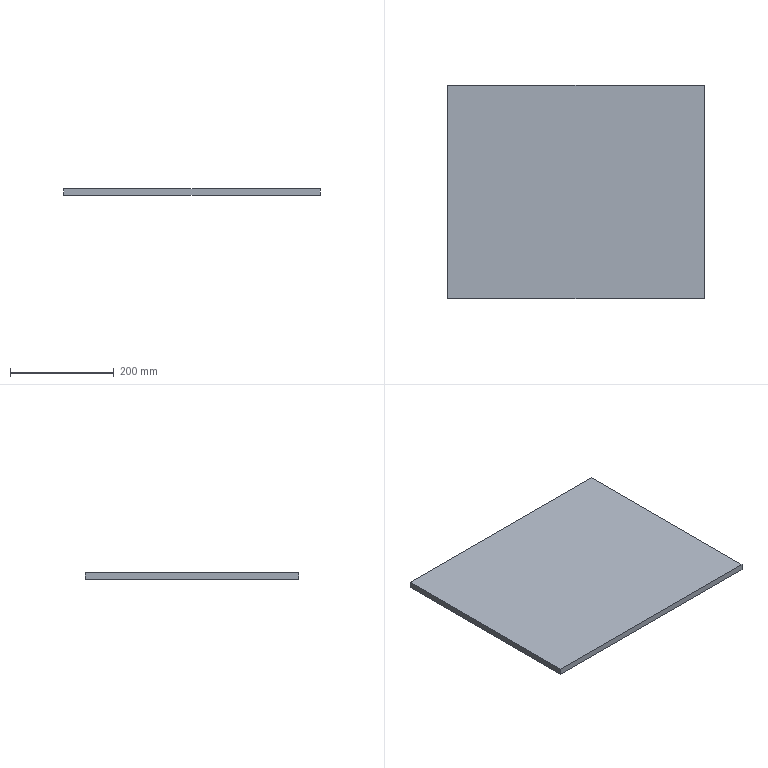Part | STEP file | Guide rail mounting plate | 1 solid | 6 faces | box 493 x 410 x 12 mm | volume 2425560 mm3 | plane 6
STEP:
#1=CARTESIAN_POINT('',(246.5,-205.,0.));
#2=VERTEX_POINT('',#1);
#3=CARTESIAN_POINT('',(246.5,205.,0.));
#4=VERTEX_POINT('',#3);
#5=CARTESIAN_POINT('',(246.5,-205.,0.));
#6=DIRECTION('',(0.,1.,0.));
#7=VECTOR('',#6,1000.);
#8=LINE('',#5,#7);
#9=EDGE_CURVE('',#2,#4,#8,.T.);
#10=ORIENTED_EDGE('',*,*,#9,.T.);
#11=CARTESIAN_POINT('',(246.5,205.,12.));
#12=VERTEX_POINT('',#11);
#13=CARTESIAN_POINT('',(246.5,205.,12.));
#14=DIRECTION('',(0.,0.,-1.));
#15=VECTOR('',#14,1000.);
#16=LINE('',#13,#15);
#17=EDGE_CURVE('',#12,#4,#16,.T.);
#18=ORIENTED_EDGE('',*,*,#17,.F.);
#19=CARTESIAN_POINT('',(246.5,-205.,12.));
#20=VERTEX_POINT('',#19);
#21=CARTESIAN_POINT('',(246.5,-205.,12.));
#22=DIRECTION('',(0.,1.,0.));
#23=VECTOR('',#22,1000.);
#24=LINE('',#21,#23);
#25=EDGE_CURVE('',#20,#12,#24,.T.);
#26=ORIENTED_EDGE('',*,*,#25,.F.);
#27=CARTESIAN_POINT('',(246.5,-205.,12.));
#28=DIRECTION('',(0.,0.,-1.));
#29=VECTOR('',#28,1000.);
#30=LINE('',#27,#29);
#31=EDGE_CURVE('',#20,#2,#30,.T.);
#32=ORIENTED_EDGE('',*,*,#31,.T.);
#33=EDGE_LOOP('',(#10,#18,#26,#32));
#34=FACE_OUTER_BOUND('',#33,.T.);
#35=CARTESIAN_POINT('',(246.5,-205.,12.));
#36=DIRECTION('',(-1.,0.,0.));
#37=DIRECTION('',(0.,0.,1.));
#38=AXIS2_PLACEMENT_3D('',#35,#36,#37);
#39=PLANE('',#38);
#40=ADVANCED_FACE('',(#34),#39,.F.);
#41=CARTESIAN_POINT('',(-246.5,205.,0.));
#42=VERTEX_POINT('',#41);
#43=CARTESIAN_POINT('',(-246.5,205.,0.));
#44=DIRECTION('',(-1.,0.,0.));
#45=VECTOR('',#44,1000.);
#46=LINE('',#43,#45);
#47=EDGE_CURVE('',#4,#42,#46,.T.);
#48=ORIENTED_EDGE('',*,*,#47,.T.);
#49=CARTESIAN_POINT('',(-246.5,205.,12.));
#50=VERTEX_POINT('',#49);
#51=CARTESIAN_POINT('',(-246.5,205.,12.));
#52=DIRECTION('',(0.,0.,-1.));
#53=VECTOR('',#52,1000.);
#54=LINE('',#51,#53);
#55=EDGE_CURVE('',#50,#42,#54,.T.);
#56=ORIENTED_EDGE('',*,*,#55,.F.);
#57=CARTESIAN_POINT('',(-246.5,205.,12.));
#58=DIRECTION('',(-1.,0.,0.));
#59=VECTOR('',#58,1000.);
#60=LINE('',#57,#59);
#61=EDGE_CURVE('',#12,#50,#60,.T.);
#62=ORIENTED_EDGE('',*,*,#61,.F.);
#63=ORIENTED_EDGE('',*,*,#17,.T.);
#64=EDGE_LOOP('',(#48,#56,#62,#63));
#65=FACE_OUTER_BOUND('',#64,.T.);
#66=CARTESIAN_POINT('',(-246.5,205.,12.));
#67=DIRECTION('',(0.,-1.,0.));
#68=DIRECTION('',(0.,0.,-1.));
#69=AXIS2_PLACEMENT_3D('',#66,#67,#68);
#70=PLANE('',#69);
#71=ADVANCED_FACE('',(#65),#70,.F.);
#72=CARTESIAN_POINT('',(-246.5,-205.,0.));
#73=VERTEX_POINT('',#72);
#74=CARTESIAN_POINT('',(-246.5,-205.,0.));
#75=DIRECTION('',(0.,-1.,0.));
#76=VECTOR('',#75,1000.);
#77=LINE('',#74,#76);
#78=EDGE_CURVE('',#42,#73,#77,.T.);
#79=ORIENTED_EDGE('',*,*,#78,.T.);
#80=CARTESIAN_POINT('',(-246.5,-205.,12.));
#81=VERTEX_POINT('',#80);
#82=CARTESIAN_POINT('',(-246.5,-205.,12.));
#83=DIRECTION('',(0.,0.,-1.));
#84=VECTOR('',#83,1000.);
#85=LINE('',#82,#84);
#86=EDGE_CURVE('',#81,#73,#85,.T.);
#87=ORIENTED_EDGE('',*,*,#86,.F.);
#88=CARTESIAN_POINT('',(-246.5,-205.,12.));
#89=DIRECTION('',(0.,-1.,0.));
#90=VECTOR('',#89,1000.);
#91=LINE('',#88,#90);
#92=EDGE_CURVE('',#50,#81,#91,.T.);
#93=ORIENTED_EDGE('',*,*,#92,.F.);
#94=ORIENTED_EDGE('',*,*,#55,.T.);
#95=EDGE_LOOP('',(#79,#87,#93,#94));
#96=FACE_OUTER_BOUND('',#95,.T.);
#97=CARTESIAN_POINT('',(-246.5,-205.,12.));
#98=DIRECTION('',(1.,0.,0.));
#99=DIRECTION('',(0.,0.,-1.));
#100=AXIS2_PLACEMENT_3D('',#97,#98,#99);
#101=PLANE('',#100);
#102=ADVANCED_FACE('',(#96),#101,.F.);
#103=CARTESIAN_POINT('',(-246.5,-205.,0.));
#104=DIRECTION('',(1.,0.,0.));
#105=VECTOR('',#104,1000.);
#106=LINE('',#103,#105);
#107=EDGE_CURVE('',#73,#2,#106,.T.);
#108=ORIENTED_EDGE('',*,*,#107,.T.);
#109=ORIENTED_EDGE('',*,*,#31,.F.);
#110=CARTESIAN_POINT('',(-246.5,-205.,12.));
#111=DIRECTION('',(1.,0.,0.));
#112=VECTOR('',#111,1000.);
#113=LINE('',#110,#112);
#114=EDGE_CURVE('',#81,#20,#113,.T.);
#115=ORIENTED_EDGE('',*,*,#114,.F.);
#116=ORIENTED_EDGE('',*,*,#86,.T.);
#117=EDGE_LOOP('',(#108,#109,#115,#116));
#118=FACE_OUTER_BOUND('',#117,.T.);
#119=CARTESIAN_POINT('',(-246.5,-205.,12.));
#120=DIRECTION('',(0.,1.,0.));
#121=DIRECTION('',(0.,0.,1.));
#122=AXIS2_PLACEMENT_3D('',#119,#120,#121);
#123=PLANE('',#122);
#124=ADVANCED_FACE('',(#118),#123,.F.);
#125=ORIENTED_EDGE('',*,*,#25,.T.);
#126=ORIENTED_EDGE('',*,*,#61,.T.);
#127=ORIENTED_EDGE('',*,*,#92,.T.);
#128=ORIENTED_EDGE('',*,*,#114,.T.);
#129=EDGE_LOOP('',(#125,#126,#127,#128));
#130=FACE_OUTER_BOUND('',#129,.T.);
#131=CARTESIAN_POINT('',(0.,0.,12.));
#132=DIRECTION('',(0.,0.,-1.));
#133=DIRECTION('',(-1.,0.,0.));
#134=AXIS2_PLACEMENT_3D('',#131,#132,#133);
#135=PLANE('',#134);
#136=ADVANCED_FACE('',(#130),#135,.F.);
#137=ORIENTED_EDGE('',*,*,#9,.F.);
#138=ORIENTED_EDGE('',*,*,#107,.F.);
#139=ORIENTED_EDGE('',*,*,#78,.F.);
#140=ORIENTED_EDGE('',*,*,#47,.F.);
#141=EDGE_LOOP('',(#137,#138,#139,#140));
#142=FACE_OUTER_BOUND('',#141,.T.);
#143=CARTESIAN_POINT('',(0.,0.,0.));
#144=DIRECTION('',(0.,0.,-1.));
#145=DIRECTION('',(-1.,0.,0.));
#146=AXIS2_PLACEMENT_3D('',#143,#144,#145);
#147=PLANE('',#146);
#148=ADVANCED_FACE('',(#142),#147,.T.);
#149=CLOSED_SHELL('',(#40,#71,#102,#124,#136,#148));
#150=MANIFOLD_SOLID_BREP('',#149);
#151=CARTESIAN_POINT('',(0.,0.,0.));
#152=DIRECTION('',(0.,0.,1.));
#153=DIRECTION('',(1.,0.,0.));
#154=AXIS2_PLACEMENT_3D('',#151,#152,#153);
#155=(LENGTH_UNIT()NAMED_UNIT(*)SI_UNIT(.MILLI.,.METRE.));
#156=UNCERTAINTY_MEASURE_WITH_UNIT(LENGTH_MEASURE(0.00001),#155,'','');
#157=(NAMED_UNIT(*)PLANE_ANGLE_UNIT()SI_UNIT($,.RADIAN.));
#158=(NAMED_UNIT(*)SI_UNIT($,.STERADIAN.)SOLID_ANGLE_UNIT());
#159=(GEOMETRIC_REPRESENTATION_CONTEXT(3)GLOBAL_UNCERTAINTY_ASSIGNED_CONTEXT((#156))GLOBAL_UNIT_ASSIGNED_CONTEXT((#155,#157,#158))REPRESENTATION_CONTEXT('',''));
#160=ADVANCED_BREP_SHAPE_REPRESENTATION('',(#150,#154),#159);